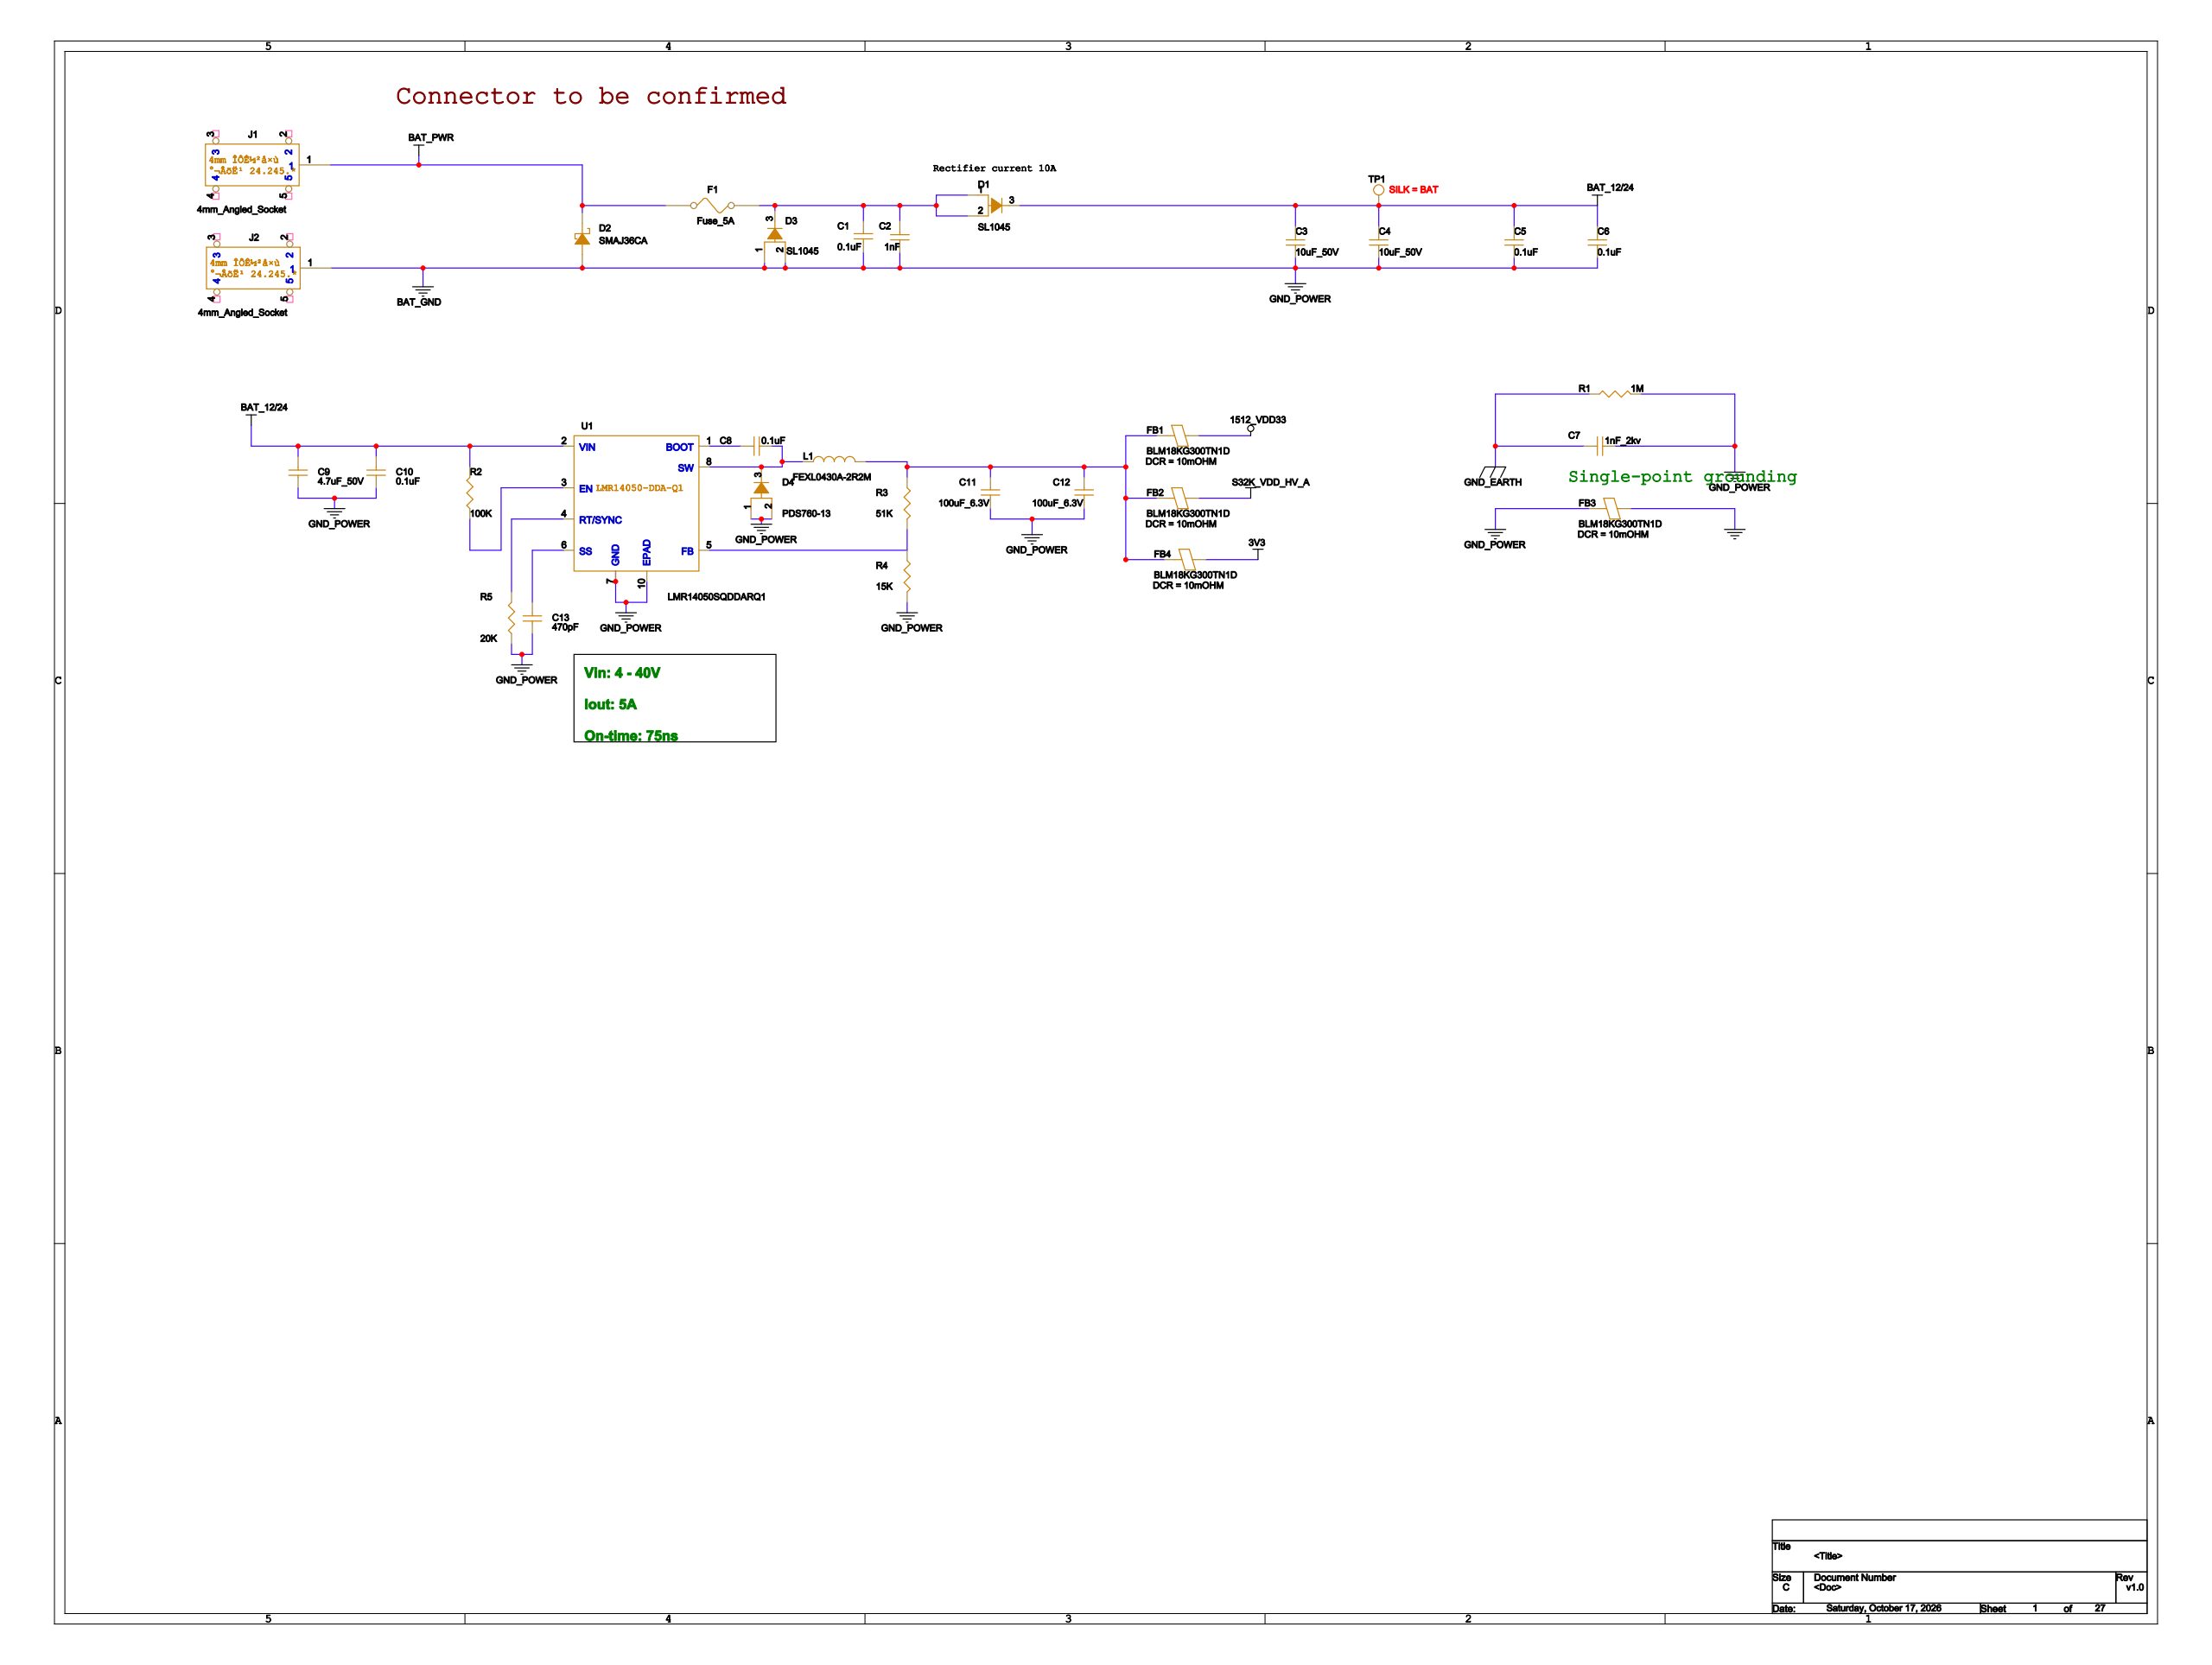Circuit board | Cadence Allegro | 477 parts | 327 nets | one sheet of the schematic
Parts on this sheet (reference | value | footprint):
C1 | 0.1uF | 0402
C2 | 1nF | 0402
C3 | 10uF_50V | 1210
C4 | 10uF_50V | 1210
C5 | 0.1uF | 0402
C6 | 0.1uF | 0402
C7 | 1nF_2kv | 1206
C8 | 0.1uF | 0402
C9 | 4.7uF_50V | 1210
C10 | 0.1uF | 0402
C11 | 100uF_6.3V | 1206
C12 | 100uF_6.3V | 1206
C13 | 470pF | 0402
D1 | SL1045 | TO277_65X40_H120
D2 | SMAJ36CA | SMAJ36
D3 | SL1045 | TO277_65X40_H120
D4 | PDS760-13 | PDS760
F1 | Fuse_5A | 1206
FB1 | BLM18KG300TN1D | 0603
FB2 | BLM18KG300TN1D | 0603
FB3 | BLM18KG300TN1D | 0603
FB4 | BLM18KG300TN1D | 0603
J1 | 4mm_Angled_Socket | YJX40016A
J2 | 4mm_Angled_Socket | YJX40016A
L1 | FEXL0430A-2R2M | L_41X41_H210_BOURNS
R1 | 1M | 1206
R2 | 100K | 0402
R3 | 51K | 0402
R4 | 15K | 0402
R5 | 20K | 0402
TP1 | TP | S0400CI
U1 | LMR14050SQDDARQ1 | SOP8P_60_PAD29X21_127_H170
Nets of these parts (net: part-pin ...):
GND: FB3-1
BAT_GND: C1-2 C2-1 C3-1 C4-1 C5-1 C6-1 C7-1 C9-1 C10-1 C11-2 C12-2 C13-1 D2-2 D3-1 D3-2 D4-1 D4-2 FB3-2 J2-1 R1-2 R4-2 R5-1 U1-7 U1-10
S32K_VDD_HV_A: FB2-1
1512_VDD33: FB1-1
3V3: FB4-1
BAT_PWR: D2-1 F1-1 J1-1
BAT_12/24: C3-2 C4-2 C5-2 C6-2 C9-2 C10-2 D1-3 R2-2 TP1-1 U1-2
N16891828: C1-1 C2-2 D1-1 D1-2 D3-3 F1-2
GND_EARTH: C7-2 R1-1
N16892245: R2-1 U1-3
N16892325: R5-2 U1-4
N16892114: C11-1 C12-1 FB1-2 FB2-2 FB4-2 L1-2 R3-1
N16892344: R3-2 R4-1 U1-5
N16892144: C8-1 D4-3 L1-1 U1-8
N16892356: C13-2 U1-6
N16892142: C8-2 U1-1